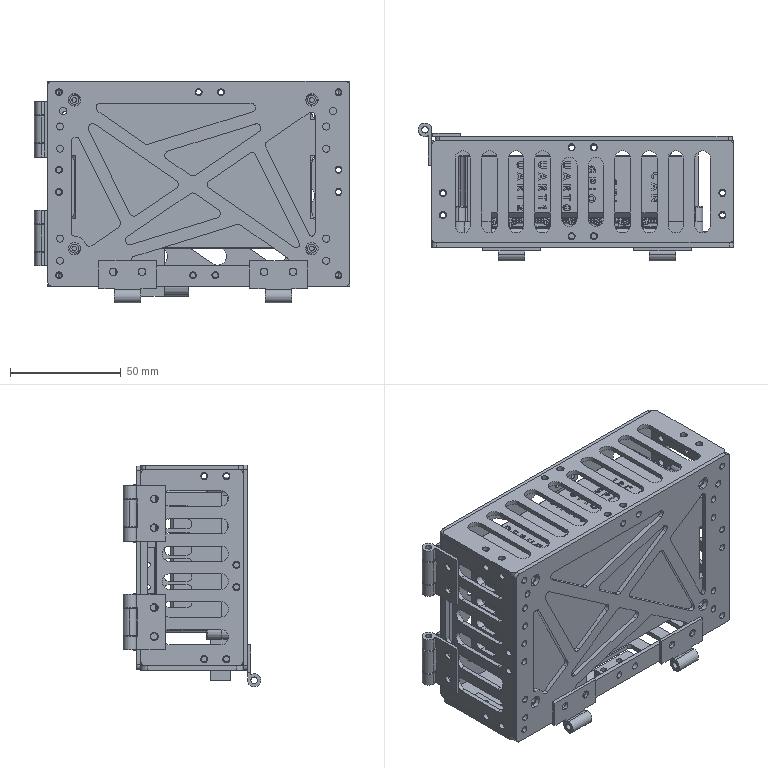Part | SolidWorks | 54 solids | 10295 faces | volume 170977 mm3 | plane 7179 | cylinder 2026 | spline 945 | cone 114 | torus 19 | sphere 12 | commonest cylinder face diameters 0.6 x202 0.3 x195 3.2 x158 2 x131 4 x127 2.5 x116